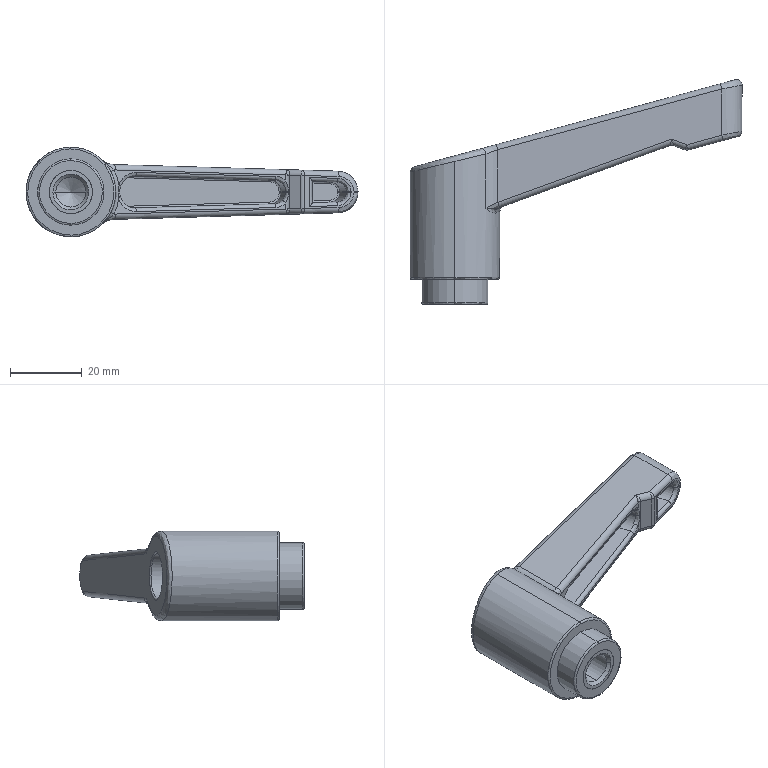Part | SolidWorks | features BaseBody 1 | 1 solid | 117 faces | box 92.5 x 62.638 x 25.001 mm | volume 27128 mm3 | cylinder 48 | spline 43 | plane 22 | cone 4 | commonest cylinder face diameters 3 x12 2 x8 1 x7 9 x3 6.6 x2 8.376 x2